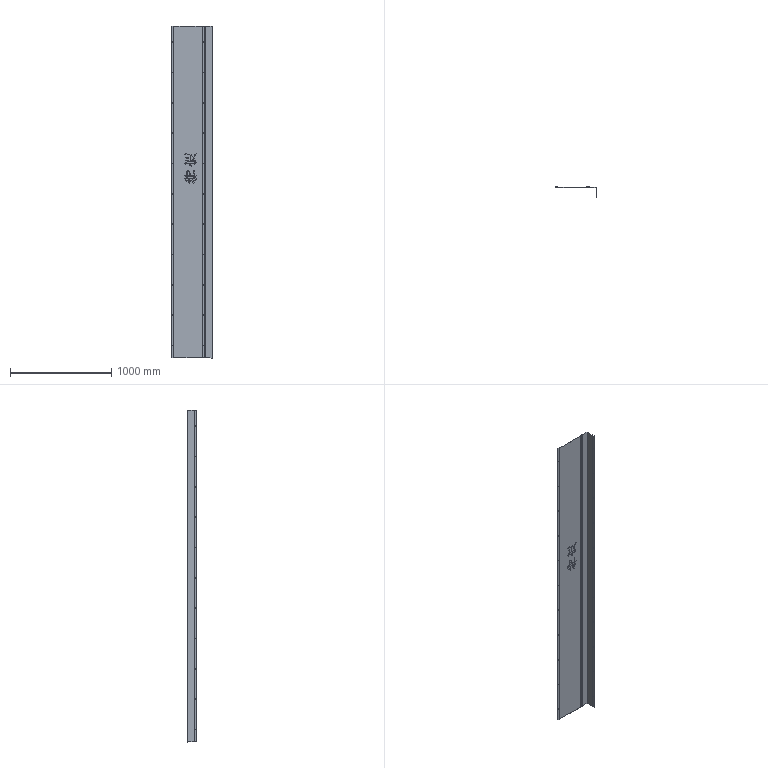Part | STEP file | TS-S36 | 1 solid | 254 faces | box 408.999 x 97.999 x 3283 mm | volume 1985800 mm3 | plane 136 | cylinder 85 | spline 33 | commonest cylinder face diameters 5.4 x66 0.4 x9 2.8 x9 10 x1